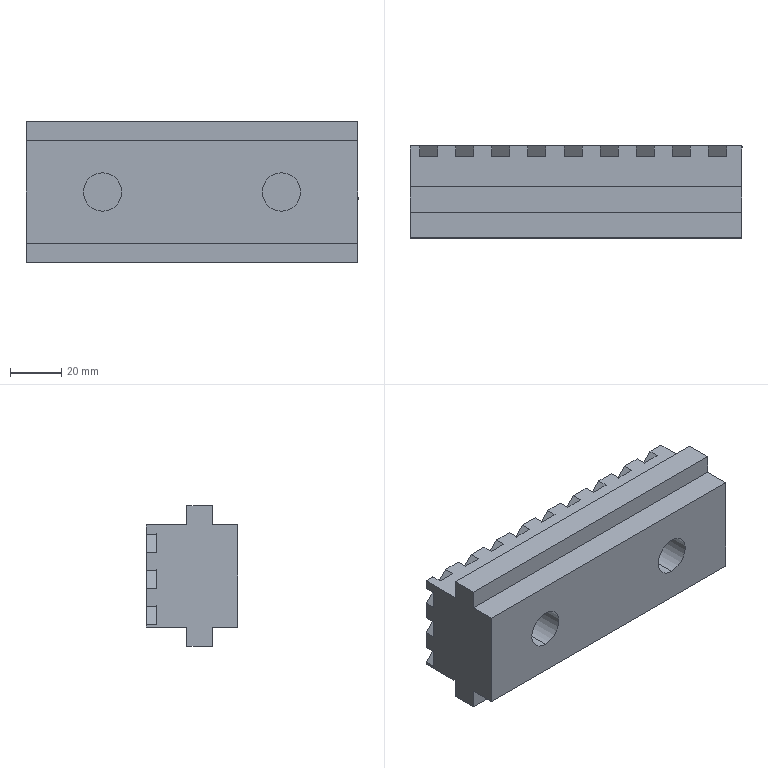Part | SolidWorks | features ICE 5, Extrusion 1 | 1 solid | 68 faces | box 130 x 36 x 55 mm | volume 187451 mm3 | plane 64 | cylinder 4 | commonest cylinder face diameters 15 x4